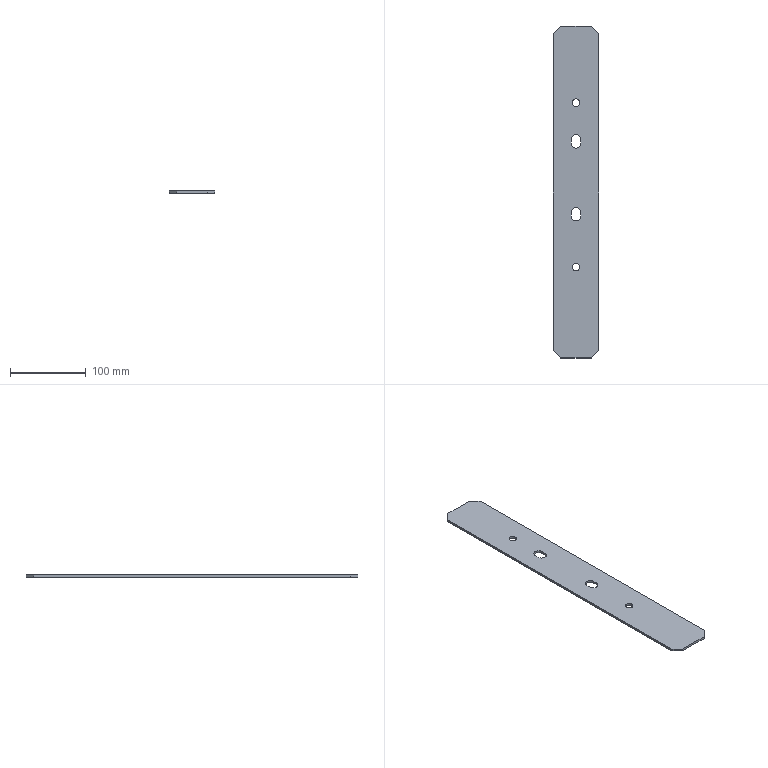Part | SolidWorks | features ICE 2, Chamfer 1, Cut 1, Extrusion 1 | 1 solid | 22 faces | box 60 x 437.5 x 3 mm | volume 76492 mm3 | plane 14 | cylinder 8 | commonest cylinder face diameters 10 x4 13 x4
STEP:
#1=CARTESIAN_POINT('',(-5.,99.,0.));
#2=VERTEX_POINT('',#1);
#3=CARTESIAN_POINT('',(5.,99.,0.));
#4=VERTEX_POINT('',#3);
#5=CARTESIAN_POINT('',(0.,99.,0.));
#6=DIRECTION('',(0.,0.,1.));
#7=DIRECTION('',(1.,0.,0.));
#8=AXIS2_PLACEMENT_3D('',#5,#6,#7);
#9=CIRCLE('',#8,5.);
#10=EDGE_CURVE('',#2,#4,#9,.T.);
#11=ORIENTED_EDGE('',*,*,#10,.F.);
#12=CARTESIAN_POINT('',(-5.,99.,3.));
#13=VERTEX_POINT('',#12);
#14=CARTESIAN_POINT('',(-5.,99.,-7.));
#15=DIRECTION('',(0.,0.,1.));
#16=VECTOR('',#15,1000.);
#17=LINE('',#14,#16);
#18=EDGE_CURVE('',#2,#13,#17,.T.);
#19=ORIENTED_EDGE('',*,*,#18,.T.);
#20=CARTESIAN_POINT('',(5.,99.,3.));
#21=VERTEX_POINT('',#20);
#22=CARTESIAN_POINT('',(0.,99.,3.));
#23=DIRECTION('',(0.,0.,1.));
#24=DIRECTION('',(1.,0.,0.));
#25=AXIS2_PLACEMENT_3D('',#22,#23,#24);
#26=CIRCLE('',#25,5.);
#27=EDGE_CURVE('',#13,#21,#26,.T.);
#28=ORIENTED_EDGE('',*,*,#27,.T.);
#29=CARTESIAN_POINT('',(5.,99.,-7.));
#30=DIRECTION('',(0.,0.,1.));
#31=VECTOR('',#30,1000.);
#32=LINE('',#29,#31);
#33=EDGE_CURVE('',#4,#21,#32,.T.);
#34=ORIENTED_EDGE('',*,*,#33,.F.);
#35=EDGE_LOOP('',(#11,#19,#28,#34));
#36=FACE_OUTER_BOUND('',#35,.T.);
#37=CARTESIAN_POINT('',(0.,99.,-7.));
#38=DIRECTION('',(0.,0.,1.));
#39=DIRECTION('',(1.,0.,0.));
#40=AXIS2_PLACEMENT_3D('',#37,#38,#39);
#41=CYLINDRICAL_SURFACE('',#40,5.);
#42=ADVANCED_FACE('',(#36),#41,.F.);
#43=CARTESIAN_POINT('',(-5.,-117.75,0.));
#44=VERTEX_POINT('',#43);
#45=CARTESIAN_POINT('',(5.,-117.75,0.));
#46=VERTEX_POINT('',#45);
#47=CARTESIAN_POINT('',(0.,-117.75,0.));
#48=DIRECTION('',(0.,0.,1.));
#49=DIRECTION('',(1.,0.,0.));
#50=AXIS2_PLACEMENT_3D('',#47,#48,#49);
#51=CIRCLE('',#50,5.);
#52=EDGE_CURVE('',#44,#46,#51,.T.);
#53=ORIENTED_EDGE('',*,*,#52,.F.);
#54=CARTESIAN_POINT('',(-5.,-117.75,3.));
#55=VERTEX_POINT('',#54);
#56=CARTESIAN_POINT('',(-5.,-117.75,-7.));
#57=DIRECTION('',(0.,0.,1.));
#58=VECTOR('',#57,1000.);
#59=LINE('',#56,#58);
#60=EDGE_CURVE('',#44,#55,#59,.T.);
#61=ORIENTED_EDGE('',*,*,#60,.T.);
#62=CARTESIAN_POINT('',(5.,-117.75,3.));
#63=VERTEX_POINT('',#62);
#64=CARTESIAN_POINT('',(0.,-117.75,3.));
#65=DIRECTION('',(0.,0.,1.));
#66=DIRECTION('',(1.,0.,0.));
#67=AXIS2_PLACEMENT_3D('',#64,#65,#66);
#68=CIRCLE('',#67,5.);
#69=EDGE_CURVE('',#55,#63,#68,.T.);
#70=ORIENTED_EDGE('',*,*,#69,.T.);
#71=CARTESIAN_POINT('',(5.,-117.75,-7.));
#72=DIRECTION('',(0.,0.,1.));
#73=VECTOR('',#72,1000.);
#74=LINE('',#71,#73);
#75=EDGE_CURVE('',#46,#63,#74,.T.);
#76=ORIENTED_EDGE('',*,*,#75,.F.);
#77=EDGE_LOOP('',(#53,#61,#70,#76));
#78=FACE_OUTER_BOUND('',#77,.T.);
#79=CARTESIAN_POINT('',(0.,-117.75,-7.));
#80=DIRECTION('',(0.,0.,1.));
#81=DIRECTION('',(1.,0.,0.));
#82=AXIS2_PLACEMENT_3D('',#79,#80,#81);
#83=CYLINDRICAL_SURFACE('',#82,5.);
#84=ADVANCED_FACE('',(#78),#83,.F.);
#85=CARTESIAN_POINT('',(30.,-227.5,3.));
#86=VERTEX_POINT('',#85);
#87=CARTESIAN_POINT('',(30.,190.,3.));
#88=VERTEX_POINT('',#87);
#89=CARTESIAN_POINT('',(30.,200.,3.));
#90=DIRECTION('',(0.,1.,0.));
#91=VECTOR('',#90,1000.);
#92=LINE('',#89,#91);
#93=EDGE_CURVE('',#86,#88,#92,.T.);
#94=ORIENTED_EDGE('',*,*,#93,.F.);
#95=CARTESIAN_POINT('',(30.,-227.5,0.));
#96=VERTEX_POINT('',#95);
#97=CARTESIAN_POINT('',(30.,-227.5,3.));
#98=DIRECTION('',(0.,0.,-1.));
#99=VECTOR('',#98,1000.);
#100=LINE('',#97,#99);
#101=EDGE_CURVE('',#86,#96,#100,.T.);
#102=ORIENTED_EDGE('',*,*,#101,.T.);
#103=CARTESIAN_POINT('',(30.,190.,0.));
#104=VERTEX_POINT('',#103);
#105=CARTESIAN_POINT('',(30.,200.,0.));
#106=DIRECTION('',(0.,1.,0.));
#107=VECTOR('',#106,1000.);
#108=LINE('',#105,#107);
#109=EDGE_CURVE('',#96,#104,#108,.T.);
#110=ORIENTED_EDGE('',*,*,#109,.T.);
#111=CARTESIAN_POINT('',(30.,190.,3.));
#112=DIRECTION('',(0.,0.,1.));
#113=VECTOR('',#112,1000.);
#114=LINE('',#111,#113);
#115=EDGE_CURVE('',#104,#88,#114,.T.);
#116=ORIENTED_EDGE('',*,*,#115,.T.);
#117=EDGE_LOOP('',(#94,#102,#110,#116));
#118=FACE_OUTER_BOUND('',#117,.T.);
#119=CARTESIAN_POINT('',(30.,200.,3.));
#120=DIRECTION('',(-1.,0.,0.));
#121=DIRECTION('',(0.,-1.,0.));
#122=AXIS2_PLACEMENT_3D('',#119,#120,#121);
#123=PLANE('',#122);
#124=ADVANCED_FACE('',(#118),#123,.F.);
#125=CARTESIAN_POINT('',(20.,200.,0.));
#126=VERTEX_POINT('',#125);
#127=CARTESIAN_POINT('',(-20.,200.,0.));
#128=VERTEX_POINT('',#127);
#129=CARTESIAN_POINT('',(-30.,200.,0.));
#130=DIRECTION('',(-1.,0.,0.));
#131=VECTOR('',#130,1000.);
#132=LINE('',#129,#131);
#133=EDGE_CURVE('',#126,#128,#132,.T.);
#134=ORIENTED_EDGE('',*,*,#133,.T.);
#135=CARTESIAN_POINT('',(-20.,200.,3.));
#136=VERTEX_POINT('',#135);
#137=CARTESIAN_POINT('',(-20.,200.,3.));
#138=DIRECTION('',(0.,0.,1.));
#139=VECTOR('',#138,1000.);
#140=LINE('',#137,#139);
#141=EDGE_CURVE('',#128,#136,#140,.T.);
#142=ORIENTED_EDGE('',*,*,#141,.T.);
#143=CARTESIAN_POINT('',(20.,200.,3.));
#144=VERTEX_POINT('',#143);
#145=CARTESIAN_POINT('',(-30.,200.,3.));
#146=DIRECTION('',(-1.,0.,0.));
#147=VECTOR('',#146,1000.);
#148=LINE('',#145,#147);
#149=EDGE_CURVE('',#144,#136,#148,.T.);
#150=ORIENTED_EDGE('',*,*,#149,.F.);
#151=CARTESIAN_POINT('',(20.,200.,3.));
#152=DIRECTION('',(0.,0.,-1.));
#153=VECTOR('',#152,1000.);
#154=LINE('',#151,#153);
#155=EDGE_CURVE('',#144,#126,#154,.T.);
#156=ORIENTED_EDGE('',*,*,#155,.T.);
#157=EDGE_LOOP('',(#134,#142,#150,#156));
#158=FACE_OUTER_BOUND('',#157,.T.);
#159=CARTESIAN_POINT('',(-30.,200.,3.));
#160=DIRECTION('',(0.,-1.,0.));
#161=DIRECTION('',(0.,0.,-1.));
#162=AXIS2_PLACEMENT_3D('',#159,#160,#161);
#163=PLANE('',#162);
#164=ADVANCED_FACE('',(#158),#163,.F.);
#165=CARTESIAN_POINT('',(-30.,190.,0.));
#166=VERTEX_POINT('',#165);
#167=CARTESIAN_POINT('',(-30.,-227.5,0.));
#168=VERTEX_POINT('',#167);
#169=CARTESIAN_POINT('',(-30.,200.,0.));
#170=DIRECTION('',(0.,-1.,0.));
#171=VECTOR('',#170,1000.);
#172=LINE('',#169,#171);
#173=EDGE_CURVE('',#166,#168,#172,.T.);
#174=ORIENTED_EDGE('',*,*,#173,.T.);
#175=CARTESIAN_POINT('',(-30.,-227.5,3.));
#176=VERTEX_POINT('',#175);
#177=CARTESIAN_POINT('',(-30.,-227.5,3.));
#178=DIRECTION('',(0.,0.,1.));
#179=VECTOR('',#178,1000.);
#180=LINE('',#177,#179);
#181=EDGE_CURVE('',#168,#176,#180,.T.);
#182=ORIENTED_EDGE('',*,*,#181,.T.);
#183=CARTESIAN_POINT('',(-30.,190.,3.));
#184=VERTEX_POINT('',#183);
#185=CARTESIAN_POINT('',(-30.,200.,3.));
#186=DIRECTION('',(0.,-1.,0.));
#187=VECTOR('',#186,1000.);
#188=LINE('',#185,#187);
#189=EDGE_CURVE('',#184,#176,#188,.T.);
#190=ORIENTED_EDGE('',*,*,#189,.F.);
#191=CARTESIAN_POINT('',(-30.,190.,3.));
#192=DIRECTION('',(0.,0.,-1.));
#193=VECTOR('',#192,1000.);
#194=LINE('',#191,#193);
#195=EDGE_CURVE('',#184,#166,#194,.T.);
#196=ORIENTED_EDGE('',*,*,#195,.T.);
#197=EDGE_LOOP('',(#174,#182,#190,#196));
#198=FACE_OUTER_BOUND('',#197,.T.);
#199=CARTESIAN_POINT('',(-30.,200.,3.));
#200=DIRECTION('',(1.,0.,0.));
#201=DIRECTION('',(0.,1.,0.));
#202=AXIS2_PLACEMENT_3D('',#199,#200,#201);
#203=PLANE('',#202);
#204=ADVANCED_FACE('',(#198),#203,.F.);
#205=CARTESIAN_POINT('',(-20.,-237.5,0.));
#206=VERTEX_POINT('',#205);
#207=CARTESIAN_POINT('',(20.,-237.5,0.));
#208=VERTEX_POINT('',#207);
#209=CARTESIAN_POINT('',(-30.,-237.5,0.));
#210=DIRECTION('',(1.,0.,0.));
#211=VECTOR('',#210,1000.);
#212=LINE('',#209,#211);
#213=EDGE_CURVE('',#206,#208,#212,.T.);
#214=ORIENTED_EDGE('',*,*,#213,.T.);
#215=CARTESIAN_POINT('',(20.,-237.5,3.));
#216=VERTEX_POINT('',#215);
#217=CARTESIAN_POINT('',(20.,-237.5,3.));
#218=DIRECTION('',(0.,0.,1.));
#219=VECTOR('',#218,1000.);
#220=LINE('',#217,#219);
#221=EDGE_CURVE('',#208,#216,#220,.T.);
#222=ORIENTED_EDGE('',*,*,#221,.T.);
#223=CARTESIAN_POINT('',(-20.,-237.5,3.));
#224=VERTEX_POINT('',#223);
#225=CARTESIAN_POINT('',(-30.,-237.5,3.));
#226=DIRECTION('',(1.,0.,0.));
#227=VECTOR('',#226,1000.);
#228=LINE('',#225,#227);
#229=EDGE_CURVE('',#224,#216,#228,.T.);
#230=ORIENTED_EDGE('',*,*,#229,.F.);
#231=CARTESIAN_POINT('',(-20.,-237.5,3.));
#232=DIRECTION('',(0.,0.,-1.));
#233=VECTOR('',#232,1000.);
#234=LINE('',#231,#233);
#235=EDGE_CURVE('',#224,#206,#234,.T.);
#236=ORIENTED_EDGE('',*,*,#235,.T.);
#237=EDGE_LOOP('',(#214,#222,#230,#236));
#238=FACE_OUTER_BOUND('',#237,.T.);
#239=CARTESIAN_POINT('',(-30.,-237.5,3.));
#240=DIRECTION('',(0.,1.,0.));
#241=DIRECTION('',(0.,0.,1.));
#242=AXIS2_PLACEMENT_3D('',#239,#240,#241);
#243=PLANE('',#242);
#244=ADVANCED_FACE('',(#238),#243,.F.);
#245=CARTESIAN_POINT('',(0.,99.,3.));
#246=DIRECTION('',(0.,0.,1.));
#247=DIRECTION('',(1.,0.,0.));
#248=AXIS2_PLACEMENT_3D('',#245,#246,#247);
#249=CIRCLE('',#248,5.);
#250=EDGE_CURVE('',#21,#13,#249,.T.);
#251=ORIENTED_EDGE('',*,*,#250,.F.);
#252=ORIENTED_EDGE('',*,*,#27,.F.);
#253=EDGE_LOOP('',(#251,#252));
#254=FACE_BOUND('',#253,.T.);
#255=CARTESIAN_POINT('',(6.5,-45.5,3.));
#256=VERTEX_POINT('',#255);
#257=CARTESIAN_POINT('',(-6.5,-45.5,3.));
#258=VERTEX_POINT('',#257);
#259=CARTESIAN_POINT('',(0.,-45.5,3.));
#260=DIRECTION('',(0.,0.,1.));
#261=DIRECTION('',(1.,0.,0.));
#262=AXIS2_PLACEMENT_3D('',#259,#260,#261);
#263=CIRCLE('',#262,6.5);
#264=EDGE_CURVE('',#256,#258,#263,.T.);
#265=ORIENTED_EDGE('',*,*,#264,.F.);
#266=CARTESIAN_POINT('',(6.5,-50.5,3.));
#267=VERTEX_POINT('',#266);
#268=CARTESIAN_POINT('',(6.5,-45.5,3.));
#269=DIRECTION('',(0.,1.,0.));
#270=VECTOR('',#269,1000.);
#271=LINE('',#268,#270);
#272=EDGE_CURVE('',#267,#256,#271,.T.);
#273=ORIENTED_EDGE('',*,*,#272,.F.);
#274=CARTESIAN_POINT('',(-6.5,-50.5,3.));
#275=VERTEX_POINT('',#274);
#276=CARTESIAN_POINT('',(0.,-50.5,3.));
#277=DIRECTION('',(0.,0.,1.));
#278=DIRECTION('',(1.,0.,0.));
#279=AXIS2_PLACEMENT_3D('',#276,#277,#278);
#280=CIRCLE('',#279,6.5);
#281=EDGE_CURVE('',#275,#267,#280,.T.);
#282=ORIENTED_EDGE('',*,*,#281,.F.);
#283=CARTESIAN_POINT('',(-6.5,-45.5,3.));
#284=DIRECTION('',(0.,-1.,0.));
#285=VECTOR('',#284,1000.);
#286=LINE('',#283,#285);
#287=EDGE_CURVE('',#258,#275,#286,.T.);
#288=ORIENTED_EDGE('',*,*,#287,.F.);
#289=EDGE_LOOP('',(#265,#273,#282,#288));
#290=FACE_BOUND('',#289,.T.);
#291=CARTESIAN_POINT('',(6.5,50.5,3.));
#292=VERTEX_POINT('',#291);
#293=CARTESIAN_POINT('',(-6.5,50.5,3.));
#294=VERTEX_POINT('',#293);
#295=CARTESIAN_POINT('',(0.,50.5,3.));
#296=DIRECTION('',(0.,0.,1.));
#297=DIRECTION('',(1.,0.,0.));
#298=AXIS2_PLACEMENT_3D('',#295,#296,#297);
#299=CIRCLE('',#298,6.5);
#300=EDGE_CURVE('',#292,#294,#299,.T.);
#301=ORIENTED_EDGE('',*,*,#300,.F.);
#302=CARTESIAN_POINT('',(6.5,45.5,3.));
#303=VERTEX_POINT('',#302);
#304=CARTESIAN_POINT('',(6.5,50.5,3.));
#305=DIRECTION('',(0.,1.,0.));
#306=VECTOR('',#305,1000.);
#307=LINE('',#304,#306);
#308=EDGE_CURVE('',#303,#292,#307,.T.);
#309=ORIENTED_EDGE('',*,*,#308,.F.);
#310=CARTESIAN_POINT('',(-6.5,45.5,3.));
#311=VERTEX_POINT('',#310);
#312=CARTESIAN_POINT('',(0.,45.5,3.));
#313=DIRECTION('',(0.,0.,1.));
#314=DIRECTION('',(1.,0.,0.));
#315=AXIS2_PLACEMENT_3D('',#312,#313,#314);
#316=CIRCLE('',#315,6.5);
#317=EDGE_CURVE('',#311,#303,#316,.T.);
#318=ORIENTED_EDGE('',*,*,#317,.F.);
#319=CARTESIAN_POINT('',(-6.5,50.5,3.));
#320=DIRECTION('',(0.,-1.,0.));
#321=VECTOR('',#320,1000.);
#322=LINE('',#319,#321);
#323=EDGE_CURVE('',#294,#311,#322,.T.);
#324=ORIENTED_EDGE('',*,*,#323,.F.);
#325=EDGE_LOOP('',(#301,#309,#318,#324));
#326=FACE_BOUND('',#325,.T.);
#327=CARTESIAN_POINT('',(0.,-117.75,3.));
#328=DIRECTION('',(0.,0.,1.));
#329=DIRECTION('',(1.,0.,0.));
#330=AXIS2_PLACEMENT_3D('',#327,#328,#329);
#331=CIRCLE('',#330,5.);
#332=EDGE_CURVE('',#63,#55,#331,.T.);
#333=ORIENTED_EDGE('',*,*,#332,.F.);
#334=ORIENTED_EDGE('',*,*,#69,.F.);
#335=EDGE_LOOP('',(#333,#334));
#336=FACE_BOUND('',#335,.T.);
#337=ORIENTED_EDGE('',*,*,#229,.T.);
#338=CARTESIAN_POINT('',(128.75,-128.75,3.));
#339=DIRECTION('',(0.7071,0.7071,0.));
#340=VECTOR('',#339,1000.);
#341=LINE('',#338,#340);
#342=EDGE_CURVE('',#216,#86,#341,.T.);
#343=ORIENTED_EDGE('',*,*,#342,.T.);
#344=ORIENTED_EDGE('',*,*,#93,.T.);
#345=CARTESIAN_POINT('',(110.,110.,3.));
#346=DIRECTION('',(-0.7071,0.7071,0.));
#347=VECTOR('',#346,1000.);
#348=LINE('',#345,#347);
#349=EDGE_CURVE('',#88,#144,#348,.T.);
#350=ORIENTED_EDGE('',*,*,#349,.T.);
#351=ORIENTED_EDGE('',*,*,#149,.T.);
#352=CARTESIAN_POINT('',(-110.,110.,3.));
#353=DIRECTION('',(-0.7071,-0.7071,0.));
#354=VECTOR('',#353,1000.);
#355=LINE('',#352,#354);
#356=EDGE_CURVE('',#136,#184,#355,.T.);
#357=ORIENTED_EDGE('',*,*,#356,.T.);
#358=ORIENTED_EDGE('',*,*,#189,.T.);
#359=CARTESIAN_POINT('',(-128.75,-128.75,3.));
#360=DIRECTION('',(0.7071,-0.7071,0.));
#361=VECTOR('',#360,1000.);
#362=LINE('',#359,#361);
#363=EDGE_CURVE('',#176,#224,#362,.T.);
#364=ORIENTED_EDGE('',*,*,#363,.T.);
#365=EDGE_LOOP('',(#337,#343,#344,#350,#351,#357,#358,#364));
#366=FACE_OUTER_BOUND('',#365,.T.);
#367=CARTESIAN_POINT('',(0.,0.,3.));
#368=DIRECTION('',(0.,0.,1.));
#369=DIRECTION('',(1.,0.,0.));
#370=AXIS2_PLACEMENT_3D('',#367,#368,#369);
#371=PLANE('',#370);
#372=ADVANCED_FACE('',(#254,#290,#326,#336,#366),#371,.T.);
#373=CARTESIAN_POINT('',(0.,99.,0.));
#374=DIRECTION('',(0.,0.,1.));
#375=DIRECTION('',(1.,0.,0.));
#376=AXIS2_PLACEMENT_3D('',#373,#374,#375);
#377=CIRCLE('',#376,5.);
#378=EDGE_CURVE('',#4,#2,#377,.T.);
#379=ORIENTED_EDGE('',*,*,#378,.T.);
#380=ORIENTED_EDGE('',*,*,#10,.T.);
#381=EDGE_LOOP('',(#379,#380));
#382=FACE_BOUND('',#381,.T.);
#383=CARTESIAN_POINT('',(6.5,-50.5,0.));
#384=VERTEX_POINT('',#383);
#385=CARTESIAN_POINT('',(6.5,-45.5,0.));
#386=VERTEX_POINT('',#385);
#387=CARTESIAN_POINT('',(6.5,0.,0.));
#388=DIRECTION('',(0.,1.,0.));
#389=VECTOR('',#388,1000.);
#390=LINE('',#387,#389);
#391=EDGE_CURVE('',#384,#386,#390,.T.);
#392=ORIENTED_EDGE('',*,*,#391,.T.);
#393=CARTESIAN_POINT('',(-6.5,-45.5,0.));
#394=VERTEX_POINT('',#393);
#395=CARTESIAN_POINT('',(0.,-45.5,0.));
#396=DIRECTION('',(0.,0.,1.));
#397=DIRECTION('',(1.,0.,0.));
#398=AXIS2_PLACEMENT_3D('',#395,#396,#397);
#399=CIRCLE('',#398,6.5);
#400=EDGE_CURVE('',#386,#394,#399,.T.);
#401=ORIENTED_EDGE('',*,*,#400,.T.);
#402=CARTESIAN_POINT('',(-6.5,-50.5,0.));
#403=VERTEX_POINT('',#402);
#404=CARTESIAN_POINT('',(-6.5,0.,0.));
#405=DIRECTION('',(0.,-1.,0.));
#406=VECTOR('',#405,1000.);
#407=LINE('',#404,#406);
#408=EDGE_CURVE('',#394,#403,#407,.T.);
#409=ORIENTED_EDGE('',*,*,#408,.T.);
#410=CARTESIAN_POINT('',(0.,-50.5,0.));
#411=DIRECTION('',(0.,0.,1.));
#412=DIRECTION('',(1.,0.,0.));
#413=AXIS2_PLACEMENT_3D('',#410,#411,#412);
#414=CIRCLE('',#413,6.5);
#415=EDGE_CURVE('',#403,#384,#414,.T.);
#416=ORIENTED_EDGE('',*,*,#415,.T.);
#417=EDGE_LOOP('',(#392,#401,#409,#416));
#418=FACE_BOUND('',#417,.T.);
#419=CARTESIAN_POINT('',(6.5,45.5,0.));
#420=VERTEX_POINT('',#419);
#421=CARTESIAN_POINT('',(6.5,50.5,0.));
#422=VERTEX_POINT('',#421);
#423=CARTESIAN_POINT('',(6.5,0.,0.));
#424=DIRECTION('',(0.,1.,0.));
#425=VECTOR('',#424,1000.);
#426=LINE('',#423,#425);
#427=EDGE_CURVE('',#420,#422,#426,.T.);
#428=ORIENTED_EDGE('',*,*,#427,.T.);
#429=CARTESIAN_POINT('',(-6.5,50.5,0.));
#430=VERTEX_POINT('',#429);
#431=CARTESIAN_POINT('',(0.,50.5,0.));
#432=DIRECTION('',(0.,0.,1.));
#433=DIRECTION('',(1.,0.,0.));
#434=AXIS2_PLACEMENT_3D('',#431,#432,#433);
#435=CIRCLE('',#434,6.5);
#436=EDGE_CURVE('',#422,#430,#435,.T.);
#437=ORIENTED_EDGE('',*,*,#436,.T.);
#438=CARTESIAN_POINT('',(-6.5,45.5,0.));
#439=VERTEX_POINT('',#438);
#440=CARTESIAN_POINT('',(-6.5,0.,0.));
#441=DIRECTION('',(0.,-1.,0.));
#442=VECTOR('',#441,1000.);
#443=LINE('',#440,#442);
#444=EDGE_CURVE('',#430,#439,#443,.T.);
#445=ORIENTED_EDGE('',*,*,#444,.T.);
#446=CARTESIAN_POINT('',(0.,45.5,0.));
#447=DIRECTION('',(0.,0.,1.));
#448=DIRECTION('',(1.,0.,0.));
#449=AXIS2_PLACEMENT_3D('',#446,#447,#448);
#450=CIRCLE('',#449,6.5);
#451=EDGE_CURVE('',#439,#420,#450,.T.);
#452=ORIENTED_EDGE('',*,*,#451,.T.);
#453=EDGE_LOOP('',(#428,#437,#445,#452));
#454=FACE_BOUND('',#453,.T.);
#455=CARTESIAN_POINT('',(0.,-117.75,0.));
#456=DIRECTION('',(0.,0.,1.));
#457=DIRECTION('',(1.,0.,0.));
#458=AXIS2_PLACEMENT_3D('',#455,#456,#457);
#459=CIRCLE('',#458,5.);
#460=EDGE_CURVE('',#46,#44,#459,.T.);
#461=ORIENTED_EDGE('',*,*,#460,.T.);
#462=ORIENTED_EDGE('',*,*,#52,.T.);
#463=EDGE_LOOP('',(#461,#462));
#464=FACE_BOUND('',#463,.T.);
#465=ORIENTED_EDGE('',*,*,#109,.F.);
#466=CARTESIAN_POINT('',(30.,-227.5,0.));
#467=DIRECTION('',(-0.7071,-0.7071,0.));
#468=VECTOR('',#467,1000.);
#469=LINE('',#466,#468);
#470=EDGE_CURVE('',#96,#208,#469,.T.);
#471=ORIENTED_EDGE('',*,*,#470,.T.);
#472=ORIENTED_EDGE('',*,*,#213,.F.);
#473=CARTESIAN_POINT('',(-20.,-237.5,0.));
#474=DIRECTION('',(-0.7071,0.7071,0.));
#475=VECTOR('',#474,1000.);
#476=LINE('',#473,#475);
#477=EDGE_CURVE('',#206,#168,#476,.T.);
#478=ORIENTED_EDGE('',*,*,#477,.T.);
#479=ORIENTED_EDGE('',*,*,#173,.F.);
#480=CARTESIAN_POINT('',(-30.,190.,0.));
#481=DIRECTION('',(0.7071,0.7071,0.));
#482=VECTOR('',#481,1000.);
#483=LINE('',#480,#482);
#484=EDGE_CURVE('',#166,#128,#483,.T.);
#485=ORIENTED_EDGE('',*,*,#484,.T.);
#486=ORIENTED_EDGE('',*,*,#133,.F.);
#487=CARTESIAN_POINT('',(20.,200.,0.));
#488=DIRECTION('',(0.7071,-0.7071,0.));
#489=VECTOR('',#488,1000.);
#490=LINE('',#487,#489);
#491=EDGE_CURVE('',#126,#104,#490,.T.);
#492=ORIENTED_EDGE('',*,*,#491,.T.);
#493=EDGE_LOOP('',(#465,#471,#472,#478,#479,#485,#486,#492));
#494=FACE_OUTER_BOUND('',#493,.T.);
#495=CARTESIAN_POINT('',(0.,0.,0.));
#496=DIRECTION('',(0.,0.,1.));
#497=DIRECTION('',(1.,0.,0.));
#498=AXIS2_PLACEMENT_3D('',#495,#496,#497);
#499=PLANE('',#498);
#500=ADVANCED_FACE('',(#382,#418,#454,#464,#494),#499,.F.);
#501=ORIENTED_EDGE('',*,*,#342,.F.);
#502=ORIENTED_EDGE('',*,*,#221,.F.);
#503=ORIENTED_EDGE('',*,*,#470,.F.);
#504=ORIENTED_EDGE('',*,*,#101,.F.);
#505=EDGE_LOOP('',(#501,#502,#503,#504));
#506=FACE_OUTER_BOUND('',#505,.T.);
#507=CARTESIAN_POINT('',(30.,-227.5,3.));
#508=DIRECTION('',(-0.7071,0.7071,0.));
#509=DIRECTION('',(0.,0.,-1.));
#510=AXIS2_PLACEMENT_3D('',#507,#508,#509);
#511=PLANE('',#510);
#512=ADVANCED_FACE('',(#506),#511,.F.);
#513=ORIENTED_EDGE('',*,*,#363,.F.);
#514=ORIENTED_EDGE('',*,*,#181,.F.);
#515=ORIENTED_EDGE('',*,*,#477,.F.);
#516=ORIENTED_EDGE('',*,*,#235,.F.);
#517=EDGE_LOOP('',(#513,#514,#515,#516));
#518=FACE_OUTER_BOUND('',#517,.T.);
#519=CARTESIAN_POINT('',(-20.,-237.5,3.));
#520=DIRECTION('',(0.7071,0.7071,0.));
#521=DIRECTION('',(0.,0.,-1.));
#522=AXIS2_PLACEMENT_3D('',#519,#520,#521);
#523=PLANE('',#522);
#524=ADVANCED_FACE('',(#518),#523,.F.);
#525=ORIENTED_EDGE('',*,*,#356,.F.);
#526=ORIENTED_EDGE('',*,*,#141,.F.);
#527=ORIENTED_EDGE('',*,*,#484,.F.);
#528=ORIENTED_EDGE('',*,*,#195,.F.);
#529=EDGE_LOOP('',(#525,#526,#527,#528));
#530=FACE_OUTER_BOUND('',#529,.T.);
#531=CARTESIAN_POINT('',(-30.,190.,3.));
#532=DIRECTION('',(0.7071,-0.7071,0.));
#533=DIRECTION('',(0.,0.,-1.));
#534=AXIS2_PLACEMENT_3D('',#531,#532,#533);
#535=PLANE('',#534);
#536=ADVANCED_FACE('',(#530),#535,.F.);
#537=ORIENTED_EDGE('',*,*,#349,.F.);
#538=ORIENTED_EDGE('',*,*,#115,.F.);
#539=ORIENTED_EDGE('',*,*,#491,.F.);
#540=ORIENTED_EDGE('',*,*,#155,.F.);
#541=EDGE_LOOP('',(#537,#538,#539,#540));
#542=FACE_OUTER_BOUND('',#541,.T.);
#543=CARTESIAN_POINT('',(20.,200.,3.));
#544=DIRECTION('',(-0.7071,-0.7071,0.));
#545=DIRECTION('',(0.,0.,-1.));
#546=AXIS2_PLACEMENT_3D('',#543,#544,#545);
#547=PLANE('',#546);
#548=ADVANCED_FACE('',(#542),#547,.F.);
#549=ORIENTED_EDGE('',*,*,#60,.F.);
#550=ORIENTED_EDGE('',*,*,#460,.F.);
#551=ORIENTED_EDGE('',*,*,#75,.T.);
#552=ORIENTED_EDGE('',*,*,#332,.T.);
#553=EDGE_LOOP('',(#549,#550,#551,#552));
#554=FACE_OUTER_BOUND('',#553,.T.);
#555=CARTESIAN_POINT('',(0.,-117.75,-7.));
#556=DIRECTION('',(0.,0.,1.));
#557=DIRECTION('',(1.,0.,0.));
#558=AXIS2_PLACEMENT_3D('',#555,#556,#557);
#559=CYLINDRICAL_SURFACE('',#558,5.);
#560=ADVANCED_FACE('',(#554),#559,.F.);
#561=CARTESIAN_POINT('',(6.5,50.5,-7.));
#562=DIRECTION('',(0.,0.,1.));
#563=VECTOR('',#562,1000.);
#564=LINE('',#561,#563);
#565=EDGE_CURVE('',#422,#292,#564,.T.);
#566=ORIENTED_EDGE('',*,*,#565,.T.);
#567=ORIENTED_EDGE('',*,*,#300,.T.);
#568=CARTESIAN_POINT('',(-6.5,50.5,-7.));
#569=DIRECTION('',(0.,0.,1.));
#570=VECTOR('',#569,1000.);
#571=LINE('',#568,#570);
#572=EDGE_CURVE('',#430,#294,#571,.T.);
#573=ORIENTED_EDGE('',*,*,#572,.F.);
#574=ORIENTED_EDGE('',*,*,#436,.F.);
#575=EDGE_LOOP('',(#566,#567,#573,#574));
#576=FACE_OUTER_BOUND('',#575,.T.);
#577=CARTESIAN_POINT('',(0.,50.5,-7.));
#578=DIRECTION('',(0.,0.,1.));
#579=DIRECTION('',(1.,0.,0.));
#580=AXIS2_PLACEMENT_3D('',#577,#578,#579);
#581=CYLINDRICAL_SURFACE('',#580,6.5);
#582=ADVANCED_FACE('',(#576),#581,.F.);
#583=CARTESIAN_POINT('',(6.5,45.5,-7.));
#584=DIRECTION('',(0.,0.,1.));
#585=VECTOR('',#584,1000.);
#586=LINE('',#583,#585);
#587=EDGE_CURVE('',#420,#303,#586,.T.);
#588=ORIENTED_EDGE('',*,*,#587,.T.);
#589=ORIENTED_EDGE('',*,*,#308,.T.);
#590=ORIENTED_EDGE('',*,*,#565,.F.);
#591=ORIENTED_EDGE('',*,*,#427,.F.);
#592=EDGE_LOOP('',(#588,#589,#590,#591));
#593=FACE_OUTER_BOUND('',#592,.T.);
#594=CARTESIAN_POINT('',(6.5,50.5,-7.));
#595=DIRECTION('',(1.,0.,0.));
#596=DIRECTION('',(0.,1.,0.));
#597=AXIS2_PLACEMENT_3D('',#594,#595,#596);
#598=PLANE('',#597);
#599=ADVANCED_FACE('',(#593),#598,.F.);
#600=CARTESIAN_POINT('',(-6.5,45.5,-7.));
#601=DIRECTION('',(0.,0.,1.));
#602=VECTOR('',#601,1000.);
#603=LINE('',#600,#602);
#604=EDGE_CURVE('',#439,#311,#603,.T.);
#605=ORIENTED_EDGE('',*,*,#604,.T.);
#606=ORIENTED_EDGE('',*,*,#317,.T.);
#607=ORIENTED_EDGE('',*,*,#587,.F.);
#608=ORIENTED_EDGE('',*,*,#451,.F.);
#609=EDGE_LOOP('',(#605,#606,#607,#608));
#610=FACE_OUTER_BOUND('',#609,.T.);
#611=CARTESIAN_POINT('',(0.,45.5,-7.));
#612=DIRECTION('',(0.,0.,1.));
#613=DIRECTION('',(1.,0.,0.));
#614=AXIS2_PLACEMENT_3D('',#611,#612,#613);
#615=CYLINDRICAL_SURFACE('',#614,6.5);
#616=ADVANCED_FACE('',(#610),#615,.F.);
#617=ORIENTED_EDGE('',*,*,#572,.T.);
#618=ORIENTED_EDGE('',*,*,#323,.T.);
#619=ORIENTED_EDGE('',*,*,#604,.F.);
#620=ORIENTED_EDGE('',*,*,#444,.F.);
#621=EDGE_LOOP('',(#617,#618,#619,#620));
#622=FACE_OUTER_BOUND('',#621,.T.);
#623=CARTESIAN_POINT('',(-6.5,50.5,-7.));
#624=DIRECTION('',(-1.,0.,0.));
#625=DIRECTION('',(0.,-1.,0.));
#626=AXIS2_PLACEMENT_3D('',#623,#624,#625);
#627=PLANE('',#626);
#628=ADVANCED_FACE('',(#622),#627,.F.);
#629=CARTESIAN_POINT('',(6.5,-45.5,-7.));
#630=DIRECTION('',(0.,0.,1.));
#631=VECTOR('',#630,1000.);
#632=LINE('',#629,#631);
#633=EDGE_CURVE('',#386,#256,#632,.T.);
#634=ORIENTED_EDGE('',*,*,#633,.T.);
#635=ORIENTED_EDGE('',*,*,#264,.T.);
#636=CARTESIAN_POINT('',(-6.5,-45.5,-7.));
#637=DIRECTION('',(0.,0.,1.));
#638=VECTOR('',#637,1000.);
#639=LINE('',#636,#638);
#640=EDGE_CURVE('',#394,#258,#639,.T.);
#641=ORIENTED_EDGE('',*,*,#640,.F.);
#642=ORIENTED_EDGE('',*,*,#400,.F.);
#643=EDGE_LOOP('',(#634,#635,#641,#642));
#644=FACE_OUTER_BOUND('',#643,.T.);
#645=CARTESIAN_POINT('',(0.,-45.5,-7.));
#646=DIRECTION('',(0.,0.,1.));
#647=DIRECTION('',(1.,0.,0.));
#648=AXIS2_PLACEMENT_3D('',#645,#646,#647);
#649=CYLINDRICAL_SURFACE('',#648,6.5);
#650=ADVANCED_FACE('',(#644),#649,.F.);
#651=CARTESIAN_POINT('',(6.5,-50.5,-7.));
#652=DIRECTION('',(0.,0.,1.));
#653=VECTOR('',#652,1000.);
#654=LINE('',#651,#653);
#655=EDGE_CURVE('',#384,#267,#654,.T.);
#656=ORIENTED_EDGE('',*,*,#655,.T.);
#657=ORIENTED_EDGE('',*,*,#272,.T.);
#658=ORIENTED_EDGE('',*,*,#633,.F.);
#659=ORIENTED_EDGE('',*,*,#391,.F.);
#660=EDGE_LOOP('',(#656,#657,#658,#659));
#661=FACE_OUTER_BOUND('',#660,.T.);
#662=CARTESIAN_POINT('',(6.5,-45.5,-7.));
#663=DIRECTION('',(1.,0.,0.));
#664=DIRECTION('',(0.,0.,-1.));
#665=AXIS2_PLACEMENT_3D('',#662,#663,#664);
#666=PLANE('',#665);
#667=ADVANCED_FACE('',(#661),#666,.F.);
#668=CARTESIAN_POINT('',(-6.5,-50.5,-7.));
#669=DIRECTION('',(0.,0.,1.));
#670=VECTOR('',#669,1000.);
#671=LINE('',#668,#670);
#672=EDGE_CURVE('',#403,#275,#671,.T.);
#673=ORIENTED_EDGE('',*,*,#672,.T.);
#674=ORIENTED_EDGE('',*,*,#281,.T.);
#675=ORIENTED_EDGE('',*,*,#655,.F.);
#676=ORIENTED_EDGE('',*,*,#415,.F.);
#677=EDGE_LOOP('',(#673,#674,#675,#676));
#678=FACE_OUTER_BOUND('',#677,.T.);
#679=CARTESIAN_POINT('',(0.,-50.5,-7.));
#680=DIRECTION('',(0.,0.,1.));
#681=DIRECTION('',(1.,0.,0.));
#682=AXIS2_PLACEMENT_3D('',#679,#680,#681);
#683=CYLINDRICAL_SURFACE('',#682,6.5);
#684=ADVANCED_FACE('',(#678),#683,.F.);
#685=ORIENTED_EDGE('',*,*,#640,.T.);
#686=ORIENTED_EDGE('',*,*,#287,.T.);
#687=ORIENTED_EDGE('',*,*,#672,.F.);
#688=ORIENTED_EDGE('',*,*,#408,.F.);
#689=EDGE_LOOP('',(#685,#686,#687,#688));
#690=FACE_OUTER_BOUND('',#689,.T.);
#691=CARTESIAN_POINT('',(-6.5,-45.5,-7.));
#692=DIRECTION('',(-1.,0.,0.));
#693=DIRECTION('',(0.,-1.,0.));
#694=AXIS2_PLACEMENT_3D('',#691,#692,#693);
#695=PLANE('',#694);
#696=ADVANCED_FACE('',(#690),#695,.F.);
#697=ORIENTED_EDGE('',*,*,#18,.F.);
#698=ORIENTED_EDGE('',*,*,#378,.F.);
#699=ORIENTED_EDGE('',*,*,#33,.T.);
#700=ORIENTED_EDGE('',*,*,#250,.T.);
#701=EDGE_LOOP('',(#697,#698,#699,#700));
#702=FACE_OUTER_BOUND('',#701,.T.);
#703=CARTESIAN_POINT('',(0.,99.,-7.));
#704=DIRECTION('',(0.,0.,1.));
#705=DIRECTION('',(1.,0.,0.));
#706=AXIS2_PLACEMENT_3D('',#703,#704,#705);
#707=CYLINDRICAL_SURFACE('',#706,5.);
#708=ADVANCED_FACE('',(#702),#707,.F.);
#709=CLOSED_SHELL('',(#42,#84,#124,#164,#204,#244,#372,#500,#512,#524,#536,#548,#560,#582,#599,#616,#628,#650,#667,#684,#696,#708));
#710=MANIFOLD_SOLID_BREP('',#709);
#711=CARTESIAN_POINT('',(0.,0.,0.));
#712=DIRECTION('',(0.,0.,1.));
#713=DIRECTION('',(1.,0.,0.));
#714=AXIS2_PLACEMENT_3D('',#711,#712,#713);
#715=(LENGTH_UNIT()NAMED_UNIT(*)SI_UNIT(.MILLI.,.METRE.));
#716=UNCERTAINTY_MEASURE_WITH_UNIT(LENGTH_MEASURE(0.00001),#715,'','');
#717=(NAMED_UNIT(*)PLANE_ANGLE_UNIT()SI_UNIT($,.RADIAN.));
#718=(NAMED_UNIT(*)SI_UNIT($,.STERADIAN.)SOLID_ANGLE_UNIT());
#719=(GEOMETRIC_REPRESENTATION_CONTEXT(3)GLOBAL_UNCERTAINTY_ASSIGNED_CONTEXT((#716))GLOBAL_UNIT_ASSIGNED_CONTEXT((#715,#717,#718))REPRESENTATION_CONTEXT('',''));
#720=ADVANCED_BREP_SHAPE_REPRESENTATION('',(#710,#714),#719);